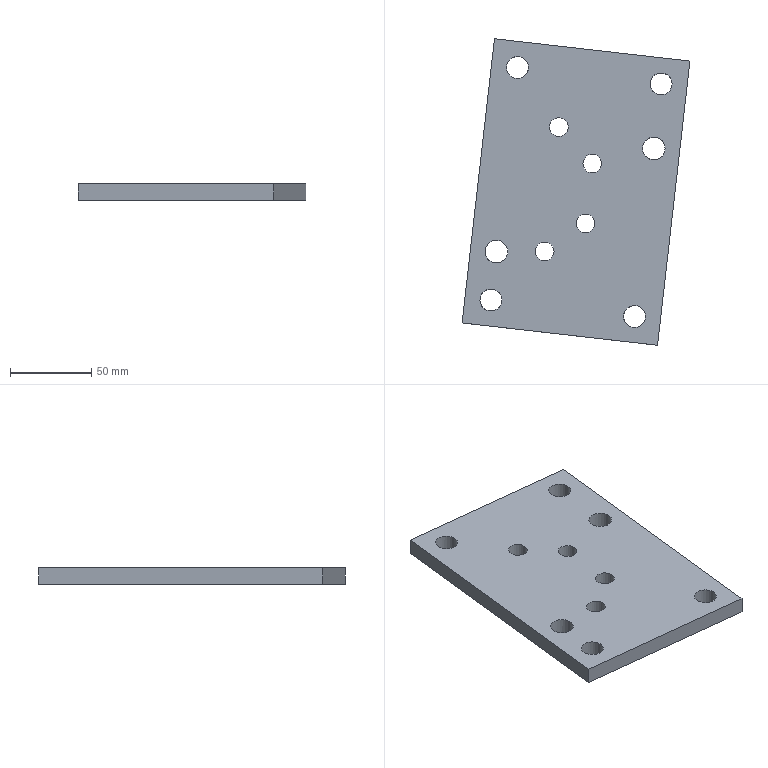Part | NX | features solid 2 | 1 solid | 16 faces | box 140.146 x 188.566 x 10 mm | volume 200000 mm3 | cylinder 10 | plane 6 | commonest cylinder face diameters 11.5 x4 13.5 x4 14.001 x2
STEP:
#1=CARTESIAN_POINT('',(2952.413,-339.568,91.));
#2=VERTEX_POINT('',#1);
#3=CARTESIAN_POINT('',(2958.163,-339.568,91.));
#4=DIRECTION('',(0.,0.,-1.));
#5=DIRECTION('',(-1.,0.,0.));
#6=AXIS2_PLACEMENT_3D('',#3,#4,#5);
#7=CIRCLE('',#6,5.75);
#8=EDGE_CURVE('',#2,#2,#7,.T.);
#9=ORIENTED_EDGE('',*,*,#8,.F.);
#10=EDGE_LOOP('',(#9));
#11=FACE_BOUND('',#10,.T.);
#12=CARTESIAN_POINT('',(2981.718,-285.538,91.));
#13=VERTEX_POINT('',#12);
#14=CARTESIAN_POINT('',(2987.468,-285.538,91.));
#15=DIRECTION('',(0.,0.,1.));
#16=DIRECTION('',(-1.,0.,0.));
#17=AXIS2_PLACEMENT_3D('',#14,#15,#16);
#18=CIRCLE('',#17,5.75);
#19=EDGE_CURVE('',#13,#13,#18,.T.);
#20=ORIENTED_EDGE('',*,*,#19,.T.);
#21=EDGE_LOOP('',(#20));
#22=FACE_BOUND('',#21,.T.);
#23=CARTESIAN_POINT('',(2935.43,-340.5,91.));
#24=VERTEX_POINT('',#23);
#25=CARTESIAN_POINT('',(2928.474,-339.708,91.));
#26=DIRECTION('',(0.,0.,1.));
#27=DIRECTION('',(0.9936,-0.1132,0.));
#28=AXIS2_PLACEMENT_3D('',#25,#26,#27);
#29=CIRCLE('',#28,7.);
#30=EDGE_CURVE('',#24,#24,#29,.T.);
#31=ORIENTED_EDGE('',*,*,#30,.T.);
#32=EDGE_LOOP('',(#31));
#33=FACE_BOUND('',#32,.T.);
#34=CARTESIAN_POINT('',(3020.212,-380.354,91.));
#35=VERTEX_POINT('',#34);
#36=CARTESIAN_POINT('',(3013.506,-379.59,91.));
#37=DIRECTION('',(0.,0.,1.));
#38=DIRECTION('',(0.9936,-0.1132,0.));
#39=AXIS2_PLACEMENT_3D('',#36,#37,#38);
#40=CIRCLE('',#39,6.75);
#41=EDGE_CURVE('',#35,#35,#40,.T.);
#42=ORIENTED_EDGE('',*,*,#41,.T.);
#43=EDGE_LOOP('',(#42));
#44=FACE_BOUND('',#43,.T.);
#45=CARTESIAN_POINT('',(2931.785,-370.279,91.));
#46=VERTEX_POINT('',#45);
#47=CARTESIAN_POINT('',(2925.078,-369.515,91.));
#48=DIRECTION('',(0.,0.,1.));
#49=DIRECTION('',(0.9936,-0.1132,0.));
#50=AXIS2_PLACEMENT_3D('',#47,#48,#49);
#51=CIRCLE('',#50,6.75);
#52=EDGE_CURVE('',#46,#46,#51,.T.);
#53=ORIENTED_EDGE('',*,*,#52,.T.);
#54=EDGE_LOOP('',(#53));
#55=FACE_BOUND('',#54,.T.);
#56=CARTESIAN_POINT('',(3027.592,-397.298,91.));
#57=VERTEX_POINT('',#56);
#58=CARTESIAN_POINT('',(3047.516,-222.43,91.));
#59=VERTEX_POINT('',#58);
#60=CARTESIAN_POINT('',(3037.554,-309.864,91.));
#61=DIRECTION('',(0.1132,0.9936,0.));
#62=VECTOR('',#61,1000.);
#63=LINE('',#60,#62);
#64=EDGE_CURVE('',#57,#59,#63,.T.);
#65=ORIENTED_EDGE('',*,*,#64,.F.);
#66=CARTESIAN_POINT('',(2907.37,-383.601,91.));
#67=VERTEX_POINT('',#66);
#68=CARTESIAN_POINT('',(2967.481,-390.449,91.));
#69=DIRECTION('',(0.9936,-0.1132,0.));
#70=VECTOR('',#69,1000.);
#71=LINE('',#68,#70);
#72=EDGE_CURVE('',#67,#57,#71,.T.);
#73=ORIENTED_EDGE('',*,*,#72,.F.);
#74=CARTESIAN_POINT('',(2927.293,-208.732,91.));
#75=VERTEX_POINT('',#74);
#76=CARTESIAN_POINT('',(2917.331,-296.166,91.));
#77=DIRECTION('',(-0.1132,-0.9936,0.));
#78=VECTOR('',#77,1000.);
#79=LINE('',#76,#78);
#80=EDGE_CURVE('',#75,#67,#79,.T.);
#81=ORIENTED_EDGE('',*,*,#80,.F.);
#82=CARTESIAN_POINT('',(2987.404,-215.581,91.));
#83=DIRECTION('',(-0.9936,0.1132,0.));
#84=VECTOR('',#83,1000.);
#85=LINE('',#82,#84);
#86=EDGE_CURVE('',#59,#75,#85,.T.);
#87=ORIENTED_EDGE('',*,*,#86,.F.);
#88=EDGE_LOOP('',(#65,#73,#81,#87));
#89=FACE_BOUND('',#88,.T.);
#90=CARTESIAN_POINT('',(3036.514,-237.28,91.));
#91=VERTEX_POINT('',#90);
#92=CARTESIAN_POINT('',(3029.807,-236.515,91.));
#93=DIRECTION('',(0.,0.,1.));
#94=DIRECTION('',(0.9936,-0.1132,0.));
#95=AXIS2_PLACEMENT_3D('',#92,#93,#94);
#96=CIRCLE('',#95,6.75);
#97=EDGE_CURVE('',#91,#91,#96,.T.);
#98=ORIENTED_EDGE('',*,*,#97,.T.);
#99=EDGE_LOOP('',(#98));
#100=FACE_BOUND('',#99,.T.);
#101=CARTESIAN_POINT('',(2948.086,-227.204,91.));
#102=VERTEX_POINT('',#101);
#103=CARTESIAN_POINT('',(2941.379,-226.44,91.));
#104=DIRECTION('',(0.,0.,1.));
#105=DIRECTION('',(0.9936,-0.1132,0.));
#106=AXIS2_PLACEMENT_3D('',#103,#104,#105);
#107=CIRCLE('',#106,6.75);
#108=EDGE_CURVE('',#102,#102,#107,.T.);
#109=ORIENTED_EDGE('',*,*,#108,.T.);
#110=EDGE_LOOP('',(#109));
#111=FACE_BOUND('',#110,.T.);
#112=CARTESIAN_POINT('',(3032.234,-277.051,91.));
#113=VERTEX_POINT('',#112);
#114=CARTESIAN_POINT('',(3025.279,-276.258,91.));
#115=DIRECTION('',(0.,0.,1.));
#116=DIRECTION('',(0.9936,-0.1132,0.));
#117=AXIS2_PLACEMENT_3D('',#114,#115,#116);
#118=CIRCLE('',#117,7.);
#119=EDGE_CURVE('',#113,#113,#118,.T.);
#120=ORIENTED_EDGE('',*,*,#119,.T.);
#121=EDGE_LOOP('',(#120));
#122=FACE_BOUND('',#121,.T.);
#123=CARTESIAN_POINT('',(2961.13,-263.063,91.));
#124=VERTEX_POINT('',#123);
#125=CARTESIAN_POINT('',(2966.88,-263.063,91.));
#126=DIRECTION('',(0.,0.,1.));
#127=DIRECTION('',(-1.,0.,0.));
#128=AXIS2_PLACEMENT_3D('',#125,#126,#127);
#129=CIRCLE('',#128,5.75);
#130=EDGE_CURVE('',#124,#124,#129,.T.);
#131=ORIENTED_EDGE('',*,*,#130,.T.);
#132=EDGE_LOOP('',(#131));
#133=FACE_BOUND('',#132,.T.);
#134=CARTESIAN_POINT('',(2977.529,-322.3,91.));
#135=VERTEX_POINT('',#134);
#136=CARTESIAN_POINT('',(2983.279,-322.3,91.));
#137=DIRECTION('',(0.,0.,1.));
#138=DIRECTION('',(-1.,0.,0.));
#139=AXIS2_PLACEMENT_3D('',#136,#137,#138);
#140=CIRCLE('',#139,5.75);
#141=EDGE_CURVE('',#135,#135,#140,.T.);
#142=ORIENTED_EDGE('',*,*,#141,.T.);
#143=EDGE_LOOP('',(#142));
#144=FACE_BOUND('',#143,.T.);
#145=CARTESIAN_POINT('',(2977.443,-303.015,91.));
#146=DIRECTION('',(0.,0.,-1.));
#147=DIRECTION('',(0.9936,-0.1132,0.));
#148=AXIS2_PLACEMENT_3D('',#145,#146,#147);
#149=PLANE('',#148);
#150=ADVANCED_FACE('',(#11,#22,#33,#44,#55,#89,#100,#111,#122,#133,#144),#149,.T.);
#151=CARTESIAN_POINT('',(2963.913,-339.568,101.));
#152=VERTEX_POINT('',#151);
#153=CARTESIAN_POINT('',(2958.163,-339.568,101.));
#154=DIRECTION('',(0.,0.,1.));
#155=DIRECTION('',(1.,0.,0.));
#156=AXIS2_PLACEMENT_3D('',#153,#154,#155);
#157=CIRCLE('',#156,5.75);
#158=EDGE_CURVE('',#152,#152,#157,.T.);
#159=ORIENTED_EDGE('',*,*,#158,.F.);
#160=EDGE_LOOP('',(#159));
#161=FACE_BOUND('',#160,.T.);
#162=CARTESIAN_POINT('',(2993.218,-285.538,101.));
#163=VERTEX_POINT('',#162);
#164=CARTESIAN_POINT('',(2987.468,-285.538,101.));
#165=DIRECTION('',(0.,0.,-1.));
#166=DIRECTION('',(1.,0.,0.));
#167=AXIS2_PLACEMENT_3D('',#164,#165,#166);
#168=CIRCLE('',#167,5.75);
#169=EDGE_CURVE('',#163,#163,#168,.T.);
#170=ORIENTED_EDGE('',*,*,#169,.T.);
#171=EDGE_LOOP('',(#170));
#172=FACE_BOUND('',#171,.T.);
#173=CARTESIAN_POINT('',(3027.592,-397.298,101.));
#174=VERTEX_POINT('',#173);
#175=CARTESIAN_POINT('',(2907.37,-383.601,101.));
#176=VERTEX_POINT('',#175);
#177=CARTESIAN_POINT('',(2967.481,-390.449,101.));
#178=DIRECTION('',(-0.9936,0.1132,0.));
#179=VECTOR('',#178,1000.);
#180=LINE('',#177,#179);
#181=EDGE_CURVE('',#174,#176,#180,.T.);
#182=ORIENTED_EDGE('',*,*,#181,.F.);
#183=CARTESIAN_POINT('',(3047.516,-222.43,101.));
#184=VERTEX_POINT('',#183);
#185=CARTESIAN_POINT('',(3037.554,-309.864,101.));
#186=DIRECTION('',(-0.1132,-0.9936,0.));
#187=VECTOR('',#186,1000.);
#188=LINE('',#185,#187);
#189=EDGE_CURVE('',#184,#174,#188,.T.);
#190=ORIENTED_EDGE('',*,*,#189,.F.);
#191=CARTESIAN_POINT('',(2927.293,-208.732,101.));
#192=VERTEX_POINT('',#191);
#193=CARTESIAN_POINT('',(2987.404,-215.581,101.));
#194=DIRECTION('',(0.9936,-0.1132,0.));
#195=VECTOR('',#194,1000.);
#196=LINE('',#193,#195);
#197=EDGE_CURVE('',#192,#184,#196,.T.);
#198=ORIENTED_EDGE('',*,*,#197,.F.);
#199=CARTESIAN_POINT('',(2917.331,-296.166,101.));
#200=DIRECTION('',(0.1132,0.9936,0.));
#201=VECTOR('',#200,1000.);
#202=LINE('',#199,#201);
#203=EDGE_CURVE('',#176,#192,#202,.T.);
#204=ORIENTED_EDGE('',*,*,#203,.F.);
#205=EDGE_LOOP('',(#182,#190,#198,#204));
#206=FACE_BOUND('',#205,.T.);
#207=CARTESIAN_POINT('',(3036.557,-236.515,101.));
#208=VERTEX_POINT('',#207);
#209=CARTESIAN_POINT('',(3029.807,-236.515,101.));
#210=DIRECTION('',(0.,0.,-1.));
#211=DIRECTION('',(1.,0.,0.));
#212=AXIS2_PLACEMENT_3D('',#209,#210,#211);
#213=CIRCLE('',#212,6.75);
#214=EDGE_CURVE('',#208,#208,#213,.T.);
#215=ORIENTED_EDGE('',*,*,#214,.T.);
#216=EDGE_LOOP('',(#215));
#217=FACE_BOUND('',#216,.T.);
#218=CARTESIAN_POINT('',(2948.129,-226.44,101.));
#219=VERTEX_POINT('',#218);
#220=CARTESIAN_POINT('',(2941.379,-226.44,101.));
#221=DIRECTION('',(0.,0.,-1.));
#222=DIRECTION('',(1.,0.,0.));
#223=AXIS2_PLACEMENT_3D('',#220,#221,#222);
#224=CIRCLE('',#223,6.75);
#225=EDGE_CURVE('',#219,#219,#224,.T.);
#226=ORIENTED_EDGE('',*,*,#225,.T.);
#227=EDGE_LOOP('',(#226));
#228=FACE_BOUND('',#227,.T.);
#229=CARTESIAN_POINT('',(3032.279,-276.258,101.));
#230=VERTEX_POINT('',#229);
#231=CARTESIAN_POINT('',(3025.279,-276.258,101.));
#232=DIRECTION('',(0.,0.,-1.));
#233=DIRECTION('',(1.,0.,0.));
#234=AXIS2_PLACEMENT_3D('',#231,#232,#233);
#235=CIRCLE('',#234,7.);
#236=EDGE_CURVE('',#230,#230,#235,.T.);
#237=ORIENTED_EDGE('',*,*,#236,.T.);
#238=EDGE_LOOP('',(#237));
#239=FACE_BOUND('',#238,.T.);
#240=CARTESIAN_POINT('',(2935.475,-339.708,101.));
#241=VERTEX_POINT('',#240);
#242=CARTESIAN_POINT('',(2928.474,-339.708,101.));
#243=DIRECTION('',(0.,0.,-1.));
#244=DIRECTION('',(1.,0.,0.));
#245=AXIS2_PLACEMENT_3D('',#242,#243,#244);
#246=CIRCLE('',#245,7.);
#247=EDGE_CURVE('',#241,#241,#246,.T.);
#248=ORIENTED_EDGE('',*,*,#247,.T.);
#249=EDGE_LOOP('',(#248));
#250=FACE_BOUND('',#249,.T.);
#251=CARTESIAN_POINT('',(3020.256,-379.59,101.));
#252=VERTEX_POINT('',#251);
#253=CARTESIAN_POINT('',(3013.506,-379.59,101.));
#254=DIRECTION('',(0.,0.,-1.));
#255=DIRECTION('',(1.,0.,0.));
#256=AXIS2_PLACEMENT_3D('',#253,#254,#255);
#257=CIRCLE('',#256,6.75);
#258=EDGE_CURVE('',#252,#252,#257,.T.);
#259=ORIENTED_EDGE('',*,*,#258,.T.);
#260=EDGE_LOOP('',(#259));
#261=FACE_BOUND('',#260,.T.);
#262=CARTESIAN_POINT('',(2931.828,-369.515,101.));
#263=VERTEX_POINT('',#262);
#264=CARTESIAN_POINT('',(2925.078,-369.515,101.));
#265=DIRECTION('',(0.,0.,-1.));
#266=DIRECTION('',(1.,0.,0.));
#267=AXIS2_PLACEMENT_3D('',#264,#265,#266);
#268=CIRCLE('',#267,6.75);
#269=EDGE_CURVE('',#263,#263,#268,.T.);
#270=ORIENTED_EDGE('',*,*,#269,.T.);
#271=EDGE_LOOP('',(#270));
#272=FACE_BOUND('',#271,.T.);
#273=CARTESIAN_POINT('',(2972.63,-263.063,101.));
#274=VERTEX_POINT('',#273);
#275=CARTESIAN_POINT('',(2966.88,-263.063,101.));
#276=DIRECTION('',(0.,0.,1.));
#277=DIRECTION('',(1.,0.,0.));
#278=AXIS2_PLACEMENT_3D('',#275,#276,#277);
#279=CIRCLE('',#278,5.75);
#280=EDGE_CURVE('',#274,#274,#279,.T.);
#281=ORIENTED_EDGE('',*,*,#280,.F.);
#282=EDGE_LOOP('',(#281));
#283=FACE_BOUND('',#282,.T.);
#284=CARTESIAN_POINT('',(2989.029,-322.3,101.));
#285=VERTEX_POINT('',#284);
#286=CARTESIAN_POINT('',(2983.279,-322.3,101.));
#287=DIRECTION('',(0.,0.,-1.));
#288=DIRECTION('',(1.,0.,0.));
#289=AXIS2_PLACEMENT_3D('',#286,#287,#288);
#290=CIRCLE('',#289,5.75);
#291=EDGE_CURVE('',#285,#285,#290,.T.);
#292=ORIENTED_EDGE('',*,*,#291,.T.);
#293=EDGE_LOOP('',(#292));
#294=FACE_BOUND('',#293,.T.);
#295=CARTESIAN_POINT('',(3398.5,0.,101.));
#296=DIRECTION('',(0.,0.,1.));
#297=DIRECTION('',(-1.,0.,0.));
#298=AXIS2_PLACEMENT_3D('',#295,#296,#297);
#299=PLANE('',#298);
#300=ADVANCED_FACE('',(#161,#172,#206,#217,#228,#239,#250,#261,#272,#283,#294),#299,.T.);
#301=CARTESIAN_POINT('',(3027.592,-397.298,91.));
#302=DIRECTION('',(0.,0.,1.));
#303=VECTOR('',#302,1000.);
#304=LINE('',#301,#303);
#305=EDGE_CURVE('',#57,#174,#304,.T.);
#306=ORIENTED_EDGE('',*,*,#305,.T.);
#307=ORIENTED_EDGE('',*,*,#181,.T.);
#308=CARTESIAN_POINT('',(2907.37,-383.601,91.));
#309=DIRECTION('',(0.,0.,1.));
#310=VECTOR('',#309,1000.);
#311=LINE('',#308,#310);
#312=EDGE_CURVE('',#67,#176,#311,.T.);
#313=ORIENTED_EDGE('',*,*,#312,.F.);
#314=ORIENTED_EDGE('',*,*,#72,.T.);
#315=EDGE_LOOP('',(#306,#307,#313,#314));
#316=FACE_BOUND('',#315,.T.);
#317=CARTESIAN_POINT('',(2967.481,-390.449,91.));
#318=DIRECTION('',(-0.1132,-0.9936,0.));
#319=DIRECTION('',(0.,0.,1.));
#320=AXIS2_PLACEMENT_3D('',#317,#318,#319);
#321=PLANE('',#320);
#322=ADVANCED_FACE('',(#316),#321,.T.);
#323=ORIENTED_EDGE('',*,*,#312,.T.);
#324=ORIENTED_EDGE('',*,*,#203,.T.);
#325=CARTESIAN_POINT('',(2927.293,-208.732,91.));
#326=DIRECTION('',(0.,0.,1.));
#327=VECTOR('',#326,1000.);
#328=LINE('',#325,#327);
#329=EDGE_CURVE('',#75,#192,#328,.T.);
#330=ORIENTED_EDGE('',*,*,#329,.F.);
#331=ORIENTED_EDGE('',*,*,#80,.T.);
#332=EDGE_LOOP('',(#323,#324,#330,#331));
#333=FACE_BOUND('',#332,.T.);
#334=CARTESIAN_POINT('',(2917.331,-296.166,91.));
#335=DIRECTION('',(-0.9936,0.1132,0.));
#336=DIRECTION('',(0.,0.,-1.));
#337=AXIS2_PLACEMENT_3D('',#334,#335,#336);
#338=PLANE('',#337);
#339=ADVANCED_FACE('',(#333),#338,.T.);
#340=ORIENTED_EDGE('',*,*,#329,.T.);
#341=ORIENTED_EDGE('',*,*,#197,.T.);
#342=CARTESIAN_POINT('',(3047.516,-222.43,91.));
#343=DIRECTION('',(0.,0.,1.));
#344=VECTOR('',#343,1000.);
#345=LINE('',#342,#344);
#346=EDGE_CURVE('',#59,#184,#345,.T.);
#347=ORIENTED_EDGE('',*,*,#346,.F.);
#348=ORIENTED_EDGE('',*,*,#86,.T.);
#349=EDGE_LOOP('',(#340,#341,#347,#348));
#350=FACE_BOUND('',#349,.T.);
#351=CARTESIAN_POINT('',(2987.404,-215.581,91.));
#352=DIRECTION('',(0.1132,0.9936,0.));
#353=DIRECTION('',(0.,0.,-1.));
#354=AXIS2_PLACEMENT_3D('',#351,#352,#353);
#355=PLANE('',#354);
#356=ADVANCED_FACE('',(#350),#355,.T.);
#357=ORIENTED_EDGE('',*,*,#346,.T.);
#358=ORIENTED_EDGE('',*,*,#189,.T.);
#359=ORIENTED_EDGE('',*,*,#305,.F.);
#360=ORIENTED_EDGE('',*,*,#64,.T.);
#361=EDGE_LOOP('',(#357,#358,#359,#360));
#362=FACE_BOUND('',#361,.T.);
#363=CARTESIAN_POINT('',(3037.554,-309.864,91.));
#364=DIRECTION('',(0.9936,-0.1132,0.));
#365=DIRECTION('',(0.,0.,1.));
#366=AXIS2_PLACEMENT_3D('',#363,#364,#365);
#367=PLANE('',#366);
#368=ADVANCED_FACE('',(#362),#367,.T.);
#369=ORIENTED_EDGE('',*,*,#52,.F.);
#370=EDGE_LOOP('',(#369));
#371=FACE_BOUND('',#370,.T.);
#372=ORIENTED_EDGE('',*,*,#269,.F.);
#373=EDGE_LOOP('',(#372));
#374=FACE_BOUND('',#373,.T.);
#375=CARTESIAN_POINT('',(2925.078,-369.515,91.));
#376=DIRECTION('',(0.,0.,1.));
#377=DIRECTION('',(-0.9936,0.1132,0.));
#378=AXIS2_PLACEMENT_3D('',#375,#376,#377);
#379=CYLINDRICAL_SURFACE('',#378,6.75);
#380=ADVANCED_FACE('',(#371,#374),#379,.F.);
#381=ORIENTED_EDGE('',*,*,#97,.F.);
#382=EDGE_LOOP('',(#381));
#383=FACE_BOUND('',#382,.T.);
#384=ORIENTED_EDGE('',*,*,#214,.F.);
#385=EDGE_LOOP('',(#384));
#386=FACE_BOUND('',#385,.T.);
#387=CARTESIAN_POINT('',(3029.807,-236.515,91.));
#388=DIRECTION('',(0.,0.,1.));
#389=DIRECTION('',(-0.9936,0.1132,0.));
#390=AXIS2_PLACEMENT_3D('',#387,#388,#389);
#391=CYLINDRICAL_SURFACE('',#390,6.75);
#392=ADVANCED_FACE('',(#383,#386),#391,.F.);
#393=ORIENTED_EDGE('',*,*,#41,.F.);
#394=EDGE_LOOP('',(#393));
#395=FACE_BOUND('',#394,.T.);
#396=ORIENTED_EDGE('',*,*,#258,.F.);
#397=EDGE_LOOP('',(#396));
#398=FACE_BOUND('',#397,.T.);
#399=CARTESIAN_POINT('',(3013.506,-379.59,91.));
#400=DIRECTION('',(0.,0.,1.));
#401=DIRECTION('',(-0.9936,0.1132,0.));
#402=AXIS2_PLACEMENT_3D('',#399,#400,#401);
#403=CYLINDRICAL_SURFACE('',#402,6.75);
#404=ADVANCED_FACE('',(#395,#398),#403,.F.);
#405=ORIENTED_EDGE('',*,*,#108,.F.);
#406=EDGE_LOOP('',(#405));
#407=FACE_BOUND('',#406,.T.);
#408=ORIENTED_EDGE('',*,*,#225,.F.);
#409=EDGE_LOOP('',(#408));
#410=FACE_BOUND('',#409,.T.);
#411=CARTESIAN_POINT('',(2941.379,-226.44,91.));
#412=DIRECTION('',(0.,0.,1.));
#413=DIRECTION('',(-0.9936,0.1132,0.));
#414=AXIS2_PLACEMENT_3D('',#411,#412,#413);
#415=CYLINDRICAL_SURFACE('',#414,6.75);
#416=ADVANCED_FACE('',(#407,#410),#415,.F.);
#417=ORIENTED_EDGE('',*,*,#30,.F.);
#418=EDGE_LOOP('',(#417));
#419=FACE_BOUND('',#418,.T.);
#420=ORIENTED_EDGE('',*,*,#247,.F.);
#421=EDGE_LOOP('',(#420));
#422=FACE_BOUND('',#421,.T.);
#423=CARTESIAN_POINT('',(2928.474,-339.708,91.));
#424=DIRECTION('',(0.,0.,1.));
#425=DIRECTION('',(-0.9936,0.1132,0.));
#426=AXIS2_PLACEMENT_3D('',#423,#424,#425);
#427=CYLINDRICAL_SURFACE('',#426,7.);
#428=ADVANCED_FACE('',(#419,#422),#427,.F.);
#429=ORIENTED_EDGE('',*,*,#119,.F.);
#430=EDGE_LOOP('',(#429));
#431=FACE_BOUND('',#430,.T.);
#432=ORIENTED_EDGE('',*,*,#236,.F.);
#433=EDGE_LOOP('',(#432));
#434=FACE_BOUND('',#433,.T.);
#435=CARTESIAN_POINT('',(3025.279,-276.258,91.));
#436=DIRECTION('',(0.,0.,1.));
#437=DIRECTION('',(-0.9936,0.1132,0.));
#438=AXIS2_PLACEMENT_3D('',#435,#436,#437);
#439=CYLINDRICAL_SURFACE('',#438,7.);
#440=ADVANCED_FACE('',(#431,#434),#439,.F.);
#441=ORIENTED_EDGE('',*,*,#19,.F.);
#442=EDGE_LOOP('',(#441));
#443=FACE_BOUND('',#442,.T.);
#444=ORIENTED_EDGE('',*,*,#169,.F.);
#445=EDGE_LOOP('',(#444));
#446=FACE_BOUND('',#445,.T.);
#447=CARTESIAN_POINT('',(2987.468,-285.538,-277.));
#448=DIRECTION('',(0.,0.,1.));
#449=DIRECTION('',(-1.,0.,0.));
#450=AXIS2_PLACEMENT_3D('',#447,#448,#449);
#451=CYLINDRICAL_SURFACE('',#450,5.75);
#452=ADVANCED_FACE('',(#443,#446),#451,.F.);
#453=ORIENTED_EDGE('',*,*,#8,.T.);
#454=EDGE_LOOP('',(#453));
#455=FACE_BOUND('',#454,.T.);
#456=ORIENTED_EDGE('',*,*,#158,.T.);
#457=EDGE_LOOP('',(#456));
#458=FACE_BOUND('',#457,.T.);
#459=CARTESIAN_POINT('',(2958.163,-339.568,-277.));
#460=DIRECTION('',(0.,0.,1.));
#461=DIRECTION('',(-1.,0.,0.));
#462=AXIS2_PLACEMENT_3D('',#459,#460,#461);
#463=CYLINDRICAL_SURFACE('',#462,5.75);
#464=ADVANCED_FACE('',(#455,#458),#463,.F.);
#465=ORIENTED_EDGE('',*,*,#130,.F.);
#466=EDGE_LOOP('',(#465));
#467=FACE_BOUND('',#466,.T.);
#468=ORIENTED_EDGE('',*,*,#280,.T.);
#469=EDGE_LOOP('',(#468));
#470=FACE_BOUND('',#469,.T.);
#471=CARTESIAN_POINT('',(2966.88,-263.063,-277.));
#472=DIRECTION('',(0.,0.,1.));
#473=DIRECTION('',(-1.,0.,0.));
#474=AXIS2_PLACEMENT_3D('',#471,#472,#473);
#475=CYLINDRICAL_SURFACE('',#474,5.75);
#476=ADVANCED_FACE('',(#467,#470),#475,.F.);
#477=ORIENTED_EDGE('',*,*,#141,.F.);
#478=EDGE_LOOP('',(#477));
#479=FACE_BOUND('',#478,.T.);
#480=ORIENTED_EDGE('',*,*,#291,.F.);
#481=EDGE_LOOP('',(#480));
#482=FACE_BOUND('',#481,.T.);
#483=CARTESIAN_POINT('',(2983.279,-322.3,-277.));
#484=DIRECTION('',(0.,0.,1.));
#485=DIRECTION('',(-1.,0.,0.));
#486=AXIS2_PLACEMENT_3D('',#483,#484,#485);
#487=CYLINDRICAL_SURFACE('',#486,5.75);
#488=ADVANCED_FACE('',(#479,#482),#487,.F.);
#489=CLOSED_SHELL('',(#150,#300,#322,#339,#356,#368,#380,#392,#404,#416,#428,#440,#452,#464,#476,#488));
#490=MANIFOLD_SOLID_BREP('',#489);
#491=(LENGTH_UNIT()NAMED_UNIT(*)SI_UNIT(.MILLI.,.METRE.));
#492=UNCERTAINTY_MEASURE_WITH_UNIT(LENGTH_MEASURE(0.00001),#491,'','');
#493=(NAMED_UNIT(*)PLANE_ANGLE_UNIT()SI_UNIT($,.RADIAN.));
#494=(NAMED_UNIT(*)SI_UNIT($,.STERADIAN.)SOLID_ANGLE_UNIT());
#495=(GEOMETRIC_REPRESENTATION_CONTEXT(3)GLOBAL_UNCERTAINTY_ASSIGNED_CONTEXT((#492))GLOBAL_UNIT_ASSIGNED_CONTEXT((#491,#493,#494))REPRESENTATION_CONTEXT('',''));
#496=ADVANCED_BREP_SHAPE_REPRESENTATION('',(#490),#495);